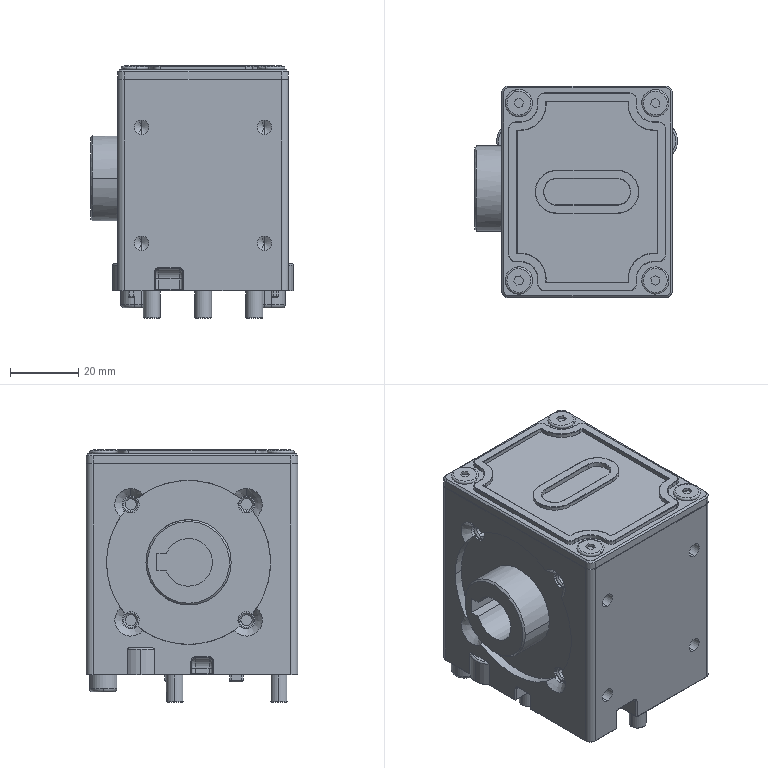Part | SolidWorks | features BaseBody 13, ICE 4, Chamfer 2 | 13 solids | 1005 faces | box 59.5 x 62 x 74 mm | volume 191803 mm3 | plane 444 | cylinder 308 | cone 177 | torus 56 | sphere 12 | spline 8 | commonest cylinder face diameters 2 x51 5 x34 1 x24 4 x24 0.2 x18 0.6 x16